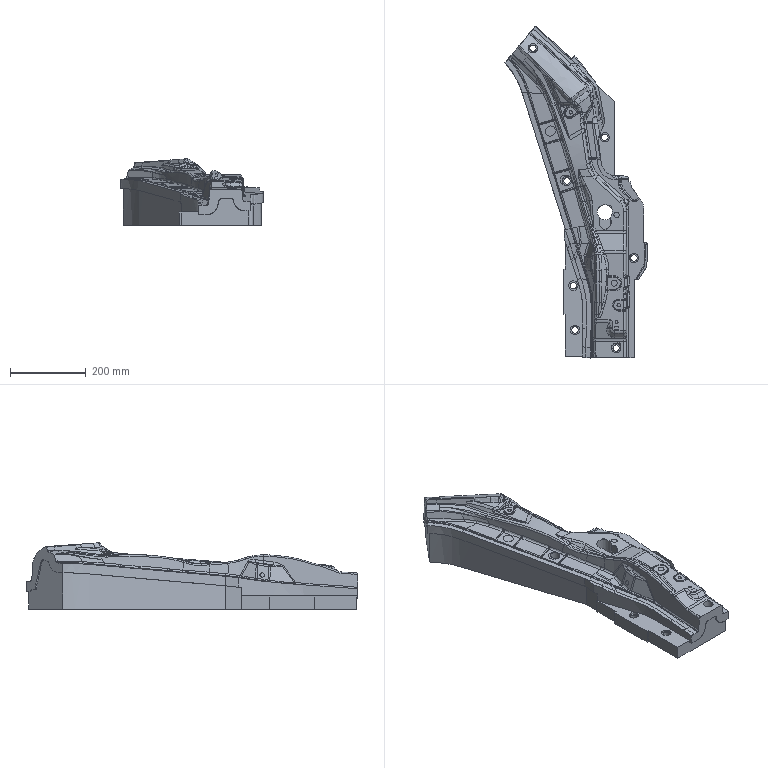Part | NX | features solid 2 | 1 solid | 704 faces | box 375.296 x 876.945 x 175.572 mm | volume 16897384 mm3 | spline 400 | cylinder 195 | plane 97 | torus 6 | sphere 5 | cone 1 | commonest cylinder face diameters 10 x52 14 x14 6 x13 20 x8 8 x7 17 x7